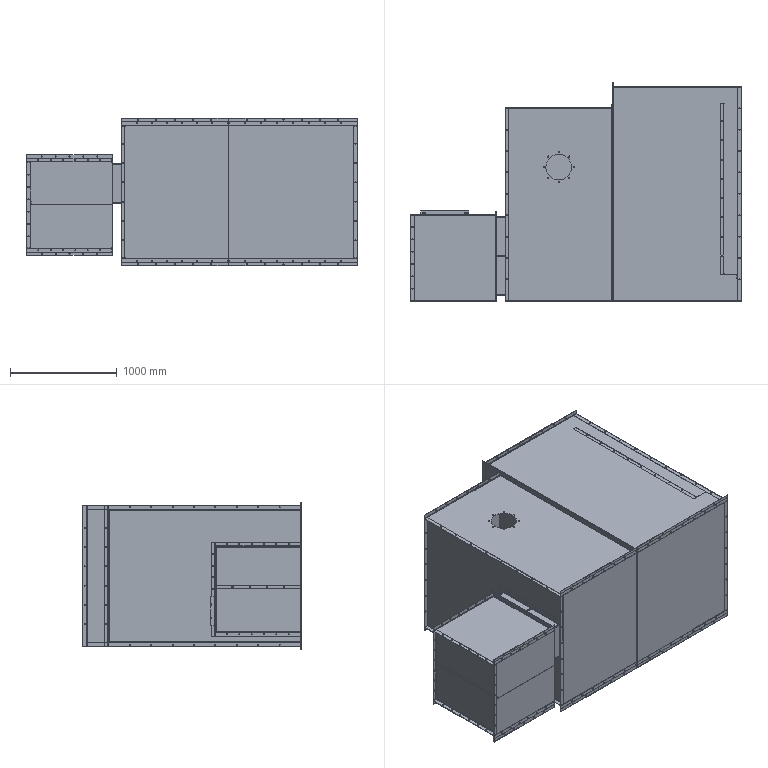Part | SolidWorks | features CompositeCurve 1 | 29 solids | 1962 faces | box 3091 x 2043 x 1380 mm | volume 102063175 mm3 | cylinder 1438 | plane 462 | spline 62 | commonest cylinder face diameters 10 x1266 12 x51 6 x47 5 x40 4.5 x8 8 x8